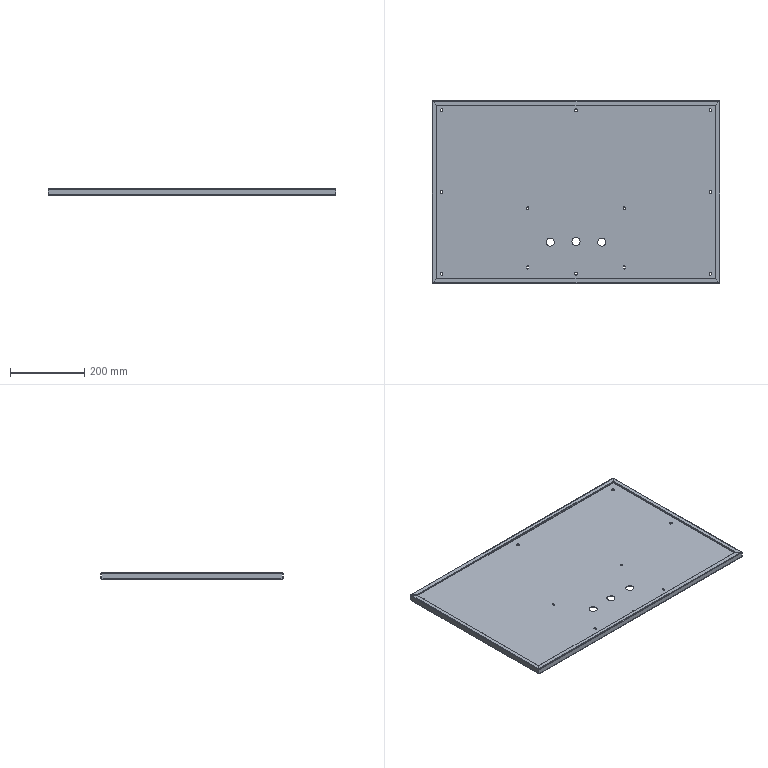Part | SolidWorks | features BaseBody 1 | 1 solid | 128 faces | box 776 x 492 x 16.5 mm | volume 663025 mm3 | plane 74 | cylinder 46 | spline 8 | commonest cylinder face diameters 7.5 x16 0.4 x8 3.4 x8 5.5 x8 22 x6